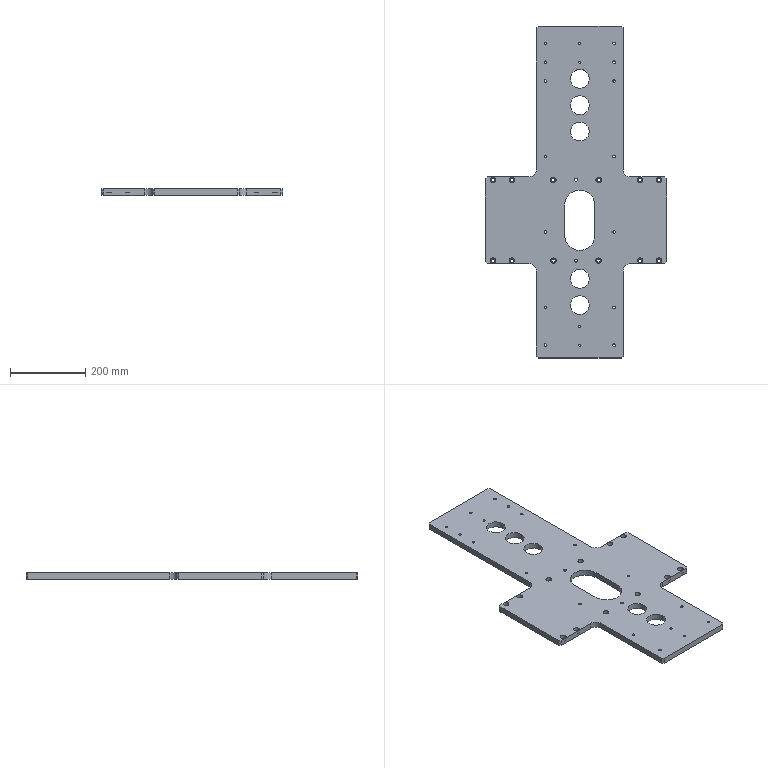Part | SolidWorks | features HoleWzd 4, Chamfer 2, Extrusion 1, Fillet 1, ICE 1 | 1 solid | 140 faces | box 480 x 880 x 16 mm | volume 3786407 mm3 | cylinder 104 | plane 36 | commonest cylinder face diameters 6.8 x28 9 x24 15 x24 50 x10 6 x8 8 x4